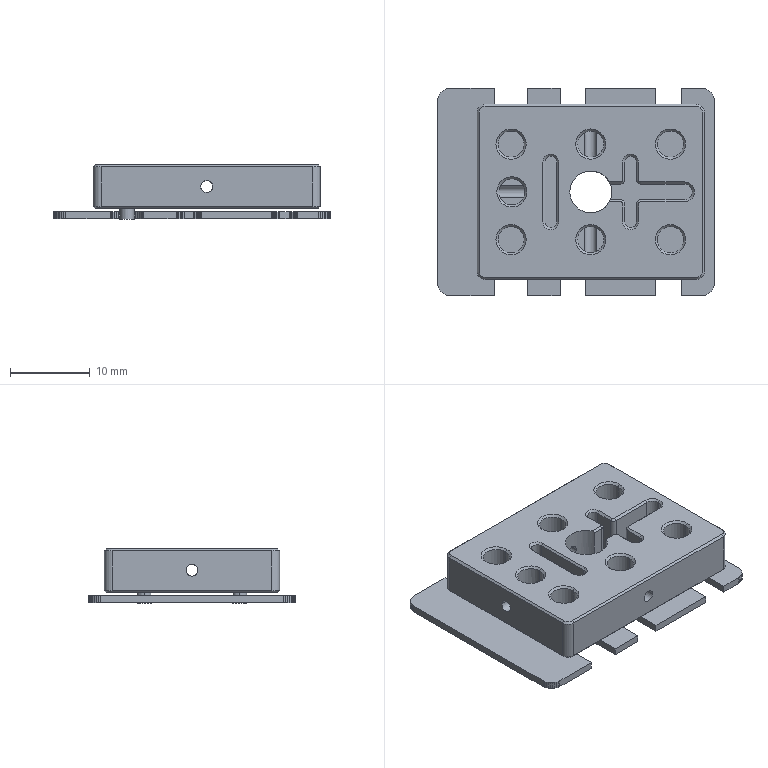Part | STEP file | 11-PCB_dwg_MODEL11 | 4 solids | 305 faces | box 34.7 x 26 x 6.86 mm | volume 3546 mm3 | plane 226 | cylinder 46 | cone 33 | commonest cylinder face diameters 1.5 x15 3.3 x14 2 x6 1 x4 1.8 x4 5.261 x3